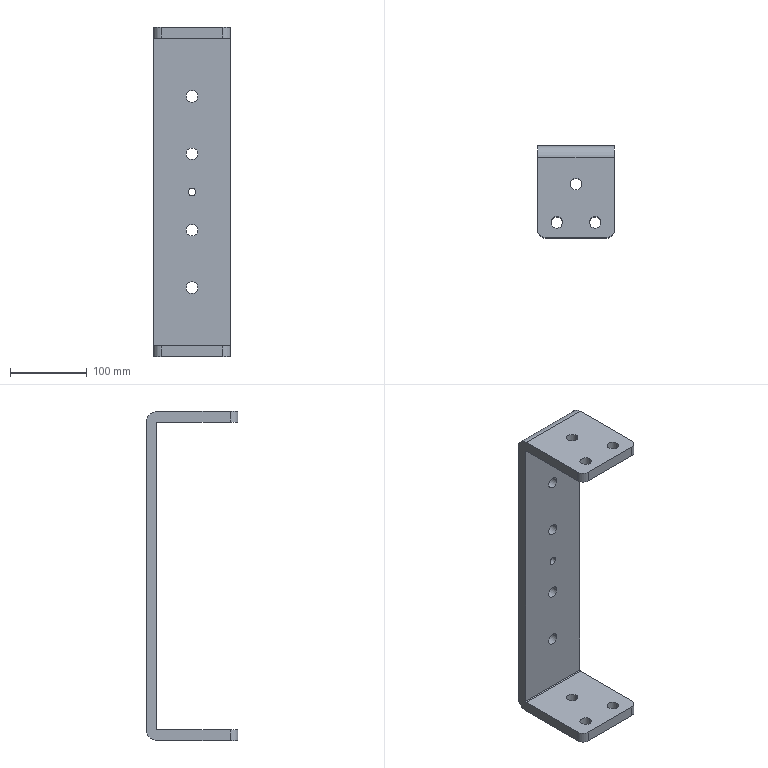Part | STEP file | Input 125 | 1 solid | 40 faces | box 100 x 120 x 430 mm | volume 862144 mm3 | cylinder 30 | plane 10 | commonest cylinder face diameters 15 x20 20 x4 2 x2 10 x2 30 x2